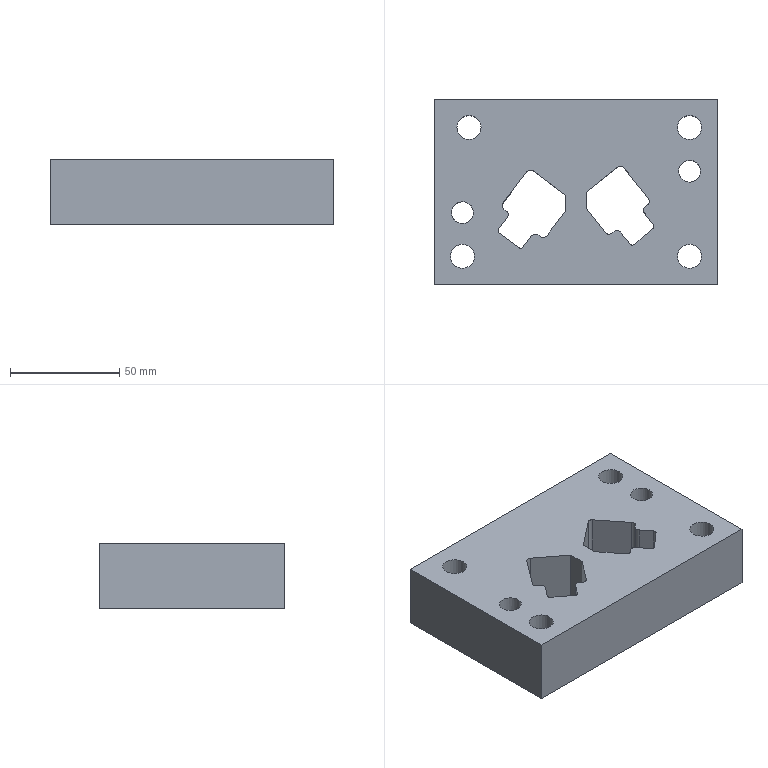Part | STEP file | 214_id702_x_t | 1 solid | 56 faces | box 130 x 85 x 30 mm | volume 266439 mm3 | plane 28 | cylinder 26 | spline 2 | commonest cylinder face diameters 4 x10 11 x6 3 x4 17 x4 10 x2